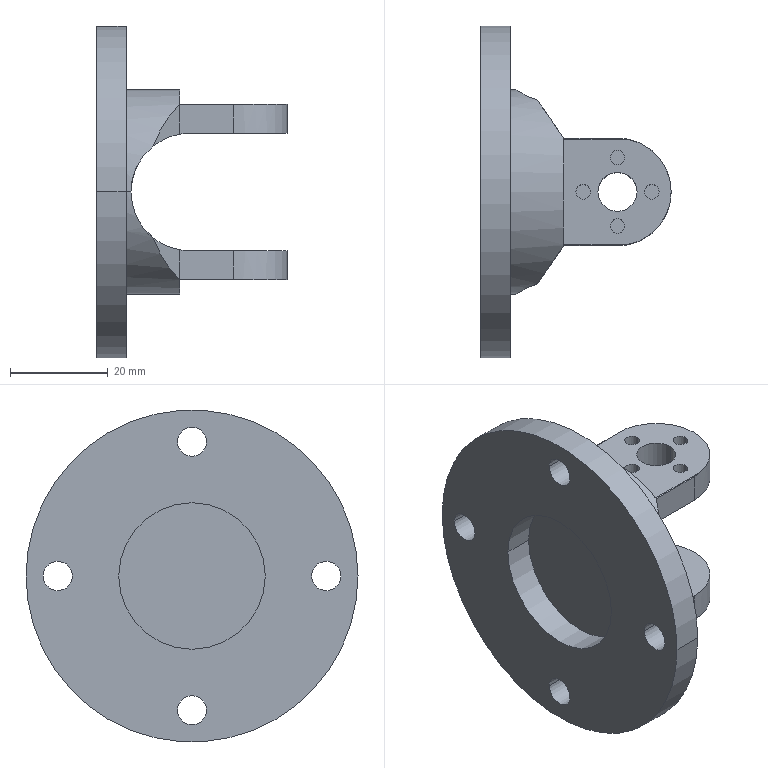Part | SolidWorks | features ICE 8, MirrorPattern 2, Revolution 1 | 1 solid | 64 faces | box 39 x 68 x 68 mm | volume 29102 mm3 | cylinder 39 | plane 25 | commonest cylinder face diameters 3 x16 6 x8 8 x4 22 x4 30 x2 42 x2